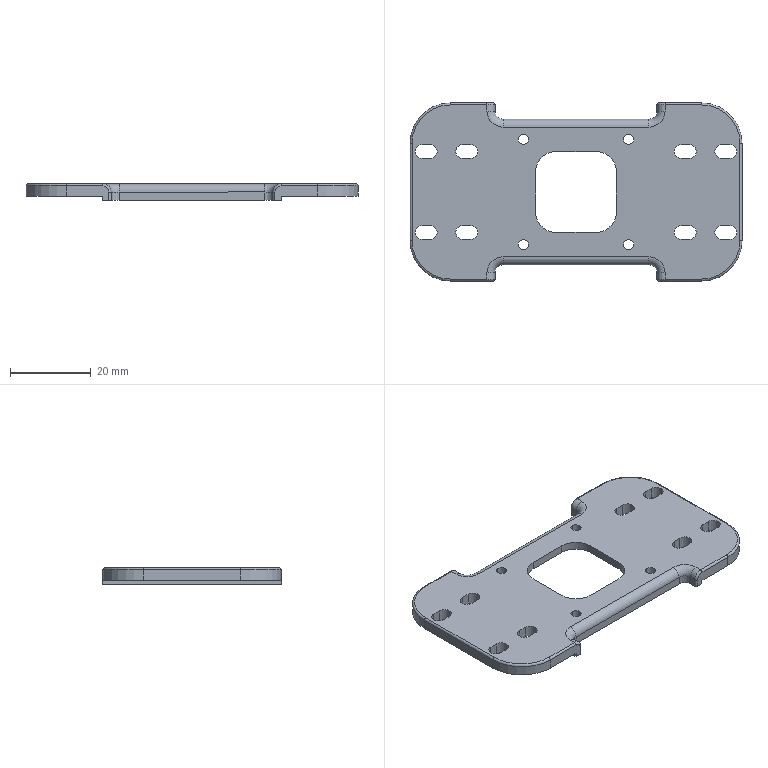NC program | NX | posted with a generic post | part box 82 x 44 x 4 mm
Lines 4216 to 5497 of 6362:
(ZLEVEL_PROFILE_1_COPY_COPY_COPY , TOOL : D3R0.5)
N8388 T18 M6
N8390 G54
N8392 G17 G0 G90 X19.987 Y23.676 S9500 M3
N8394 G43 Z30. H18
N8396 Z2.984
N8398 G94 G1 Z-0.016 F1000.
N8400 G3 X21.508 Y22.645 R1.5
N8402 G1 X22. Y22.677 F2500.
N8404 X31.
N8406 G2 X41.677 Y12. R10.677
N8408 G1 Y-12.
N8410 G2 X31. Y-22.677 R10.677
N8412 G1 X22.
N8414 X21.509 Y-22.646
N8416 X21.503 Y-22.724 Z-0.028
N8418 X21.5 Y-22.767 Z-0.04
N8420 X21.538 Y-22.762
N8422 X22. Y-22.78
N8424 X31.
N8426 G3 X41.78 Y-12. R10.78
N8428 G1 Y12.
N8430 G3 X31. Y22.78 R10.78
N8432 G1 X22.
N8434 X21.519 Y22.762
N8436 X21.509 Y22.764
N8438 X21.504 Y22.822 Z-0.057
N8440 X21.5 Y22.862 Z-0.074
N8442 X22. Y22.876
N8444 X31.
N8446 G2 X41.876 Y12. R10.876
N8448 G1 Y-12.
N8450 G2 X31. Y-22.876 R10.876
N8452 G1 X22.
N8454 X21.538 Y-22.863
N8456 X21.5 Y-22.862
N8458 Y-22.92 Z-0.095
N8460 Y-22.959 Z-0.116
N8462 X22. Y-22.968
N8464 X31.
N8466 G3 X41.968 Y-12. R10.968
N8468 G1 Y12.
N8470 G3 X31. Y22.968 R10.968
N8472 G1 X22.
N8474 X21.5 Y22.959
N8476 Y23.004 Z-0.142
N8478 Y23.049 Z-0.168
N8480 X22. Y23.055
N8482 X31.
N8484 G2 X42.055 Y12. R11.055
N8486 G1 Y-12.
N8488 G2 X31. Y-23.055 R11.055
N8490 G1 X22.
N8492 X21.5 Y-23.049
N8494 Y-23.093 Z-0.198
N8496 Y-23.127 Z-0.228
N8498 X22. Y-23.136
N8500 X31.
N8502 G3 X42.136 Y-12. R11.136
N8504 G1 Y12.
N8506 G3 X31. Y23.136 R11.136
N8508 G1 X22.
N8510 X21.5 Y23.127
N8512 Y23.168 Z-0.262
N8514 Y23.2 Z-0.296
N8516 X22. Y23.21
N8518 X31.
N8520 G2 X42.21 Y12. R11.21
N8522 G1 Y-12.
N8524 G2 X31. Y-23.21 R11.21
N8526 G1 X22.
N8528 X21.5 Y-23.2
N8530 Y-23.237 Z-0.333
N8532 Y-23.269 Z-0.37
N8534 X22. Y-23.277
N8536 X31.
N8538 G3 X42.277 Y-12. R11.277
N8540 G1 Y12.
N8542 G3 X31. Y23.277 R11.277
N8544 G1 X22.
N8546 X21.5 Y23.269
N8548 X21.416 Y23.323 Z-0.451
N8550 G2 X22. Y23.336 R15.223
N8552 G1 X31.
N8554 G2 X42.336 Y12. R11.336
N8556 G1 Y-12.
N8558 G2 X31. Y-23.336 R11.336
N8560 G1 X22.
N8562 X21.416 Y-23.325
N8564 Y-23.354 Z-0.495
N8566 Y-23.375 Z-0.538
N8568 X22. Y-23.387
N8570 X31.
N8572 G3 X42.387 Y-12. R11.387
N8574 G1 Y12.
N8576 G3 X31. Y23.387 R11.387
N8578 G1 X22.
N8580 G3 X21.416 Y23.373 R27.173
N8582 G1 Y23.4 Z-0.583
N8584 Y23.415 Z-0.629
N8586 X22. Y23.429
N8588 X31.
N8590 G2 X42.429 Y12. R11.429
N8592 G1 Y-12.
N8594 G2 X31. Y-23.429 R11.429
N8596 G1 X22.
N8598 X21.416 Y-23.417
N8600 Y-23.436 Z-0.675
N8602 Y-23.449 Z-0.722
N8604 X22. Y-23.46
N8606 X31.
N8608 G3 X42.46 Y-12. R11.46
N8610 G1 Y12.
N8612 G3 X31. Y23.46 R11.46
N8614 G1 X22.
N8616 X21.416 Y23.449
N8618 Y23.465 Z-0.768
N8620 Y23.471 Z-0.814
N8622 X22. Y23.483
N8624 X31.
N8626 G2 X42.483 Y12. R11.483
N8628 G1 Y-12.
N8630 G2 X31. Y-23.483 R11.483
N8632 G1 X22.
N8634 X21.416 Y-23.471
N8636 Y-23.481 Z-0.861
N8638 Y-23.485 Z-0.907
N8640 X22. Y-23.496
N8642 X31.
N8644 G3 X42.496 Y-12. R11.496
N8646 G1 Y12.
N8648 G3 X31. Y23.496 R11.496
N8650 G1 X22.
N8652 X21.416 Y23.485
N8654 Y23.492 Z-1.
N8656 X21.538 Y23.497
N8658 X31.055 Y23.498
N8660 G2 X42.5 Y12. R11.499
N8662 G1 Y-11.824
N8664 X42.499 Y-12.068
N8666 G2 X31.055 Y-23.498 R11.498
N8668 G1 X21.538 Y-23.497
N8670 X21.416 Y-23.492
N8672 G3 X19.883 Y-24.73 R1.5
N8674 G1 Z2.
N8676 G0 Z30.
N8678 X-20.168 Y-23.794
N8680 Z2.984
N8682 G1 Z-0.016 F1000.
N8684 X-20.991 Y-22.892
N8686 G3 X-21.51 Y-22.649 R0.75
N8688 G1 X-21.537 Y-22.663 F2500.
N8690 X-22. Y-22.677
N8692 X-31.
N8694 G2 X-41.677 Y-12. R10.677
N8696 G1 Y12.
N8698 G2 X-31. Y22.677 R10.677
N8700 G1 X-22.
N8702 X-21.508 Y22.643
N8704 Y22.705 Z-0.028
N8706 Y22.764 Z-0.04
N8708 X-21.518 Y22.761
N8710 X-22. Y22.78
N8712 X-31.
N8714 G3 X-41.78 Y12. R10.78
N8716 G1 Y-12.
N8718 G3 X-31. Y-22.78 R10.78
N8720 G1 X-22.
N8722 X-21.518 Y-22.761
N8724 X-21.508 Y-22.764
N8726 X-21.503 Y-22.822 Z-0.057
N8728 X-21.5 Y-22.862 Z-0.074
N8730 X-22. Y-22.876
N8732 X-31.
N8734 G2 X-41.876 Y-12. R10.876
N8736 G1 Y12.
N8738 G2 X-31. Y22.876 R10.876
N8740 G1 X-22.
N8742 X-21.538 Y22.863
N8744 X-21.5 Y22.862
N8746 Y22.919 Z-0.095
N8748 Y22.959 Z-0.116
N8750 X-22. Y22.968
N8752 X-31.
N8754 G3 X-41.968 Y12. R10.968
N8756 G1 Y-12.
N8758 G3 X-31. Y-22.968 R10.968
N8760 G1 X-22.
N8762 X-21.5 Y-22.959
N8764 Y-23.008 Z-0.142
N8766 Y-23.049 Z-0.168
N8768 X-22. Y-23.055
N8770 X-31.
N8772 G2 X-42.055 Y-12. R11.055
N8774 G1 Y12.
N8776 G2 X-31. Y23.055 R11.055
N8778 G1 X-22.
N8780 X-21.5 Y23.049
N8782 Y23.093 Z-0.198
N8784 Y23.127 Z-0.228
N8786 X-22. Y23.136
N8788 X-31.
N8790 G3 X-42.136 Y12. R11.136
N8792 G1 Y-12.
N8794 G3 X-31. Y-23.136 R11.136
N8796 G1 X-22.
N8798 X-21.5 Y-23.127
N8800 Y-23.168 Z-0.262
N8802 Y-23.2 Z-0.296
N8804 X-22. Y-23.21
N8806 X-31.
N8808 G2 X-42.21 Y-12. R11.21
N8810 G1 Y12.
N8812 G2 X-31. Y23.21 R11.21
N8814 G1 X-22.
N8816 X-21.5 Y23.2
N8818 Y23.237 Z-0.333
N8820 Y23.269 Z-0.37
N8822 X-22. Y23.277
N8824 X-31.
N8826 G3 X-42.277 Y12. R11.277
N8828 G1 Y-12.
N8830 G3 X-31. Y-23.277 R11.277
N8832 G1 X-22.
N8834 X-21.5 Y-23.269
N8836 Y-23.305 Z-0.411
N8838 Y-23.333 Z-0.451
N8840 X-22. Y-23.336
N8842 X-31.
N8844 G2 X-42.336 Y-12. R11.336
N8846 G1 Y12.
N8848 G2 X-31. Y23.336 R11.336
N8850 G1 X-22.
N8852 X-21.5 Y23.333
N8854 Y23.359 Z-0.495
N8856 Y23.381 Z-0.538
N8858 X-22. Y23.387
N8860 X-31.
N8862 G3 X-42.387 Y12. R11.387
N8864 G1 Y-12.
N8866 G3 X-31. Y-23.387 R11.387
N8868 G1 X-22.
N8870 X-21.5 Y-23.381
N8872 Y-23.406 Z-0.583
N8874 Y-23.424 Z-0.629
N8876 X-22. Y-23.429
N8878 X-31.
N8880 G2 X-42.429 Y-12. R11.429
N8882 G1 Y12.
N8884 G2 X-31. Y23.429 R11.429
N8886 G1 X-22.
N8888 X-21.5 Y23.424
N8890 Y23.439 Z-0.675
N8892 Y23.453 Z-0.722
N8894 X-21.538 Y23.455
N8896 X-22. Y23.46
N8898 X-31.
N8900 G3 X-42.46 Y12. R11.46
N8902 G1 Y-12.
N8904 G3 X-31. Y-23.46 R11.46
N8906 G1 X-22.
N8908 X-21.538 Y-23.455
N8910 X-21.5 Y-23.453
N8912 Y-23.47 Z-0.768
N8914 Y-23.48 Z-0.814
N8916 X-22. Y-23.483
N8918 X-31.
N8920 G2 X-42.483 Y-12. R11.483
N8922 G1 Y12.
N8924 G2 X-31. Y23.483 R11.483
N8926 G1 X-22.
N8928 X-21.474 Y23.479
N8930 X-21.416 Y23.485 Z-0.907
N8932 X-22. Y23.496
N8934 X-31.
N8936 G3 X-42.496 Y12. R11.496
N8938 G1 Y-12.
N8940 G3 X-31. Y-23.496 R11.496
N8942 G1 X-22.
N8944 X-21.416 Y-23.485
N8946 Y-23.492 Z-1.
N8948 X-21.538 Y-23.497
N8950 X-31.055 Y-23.498
N8952 G2 X-42.498 Y-12.068 R11.498
N8954 G1 Y11.998
N8956 G2 X-30.996 Y23.498 R11.501
N8958 G1 X-21.538 Y23.497
N8960 X-21.416 Y23.492
N8962 G3 X-19.876 Y24.727 R1.5
N8964 G1 Z2.
N8966 G0 Z30.
(ZLEVEL_PROFILE_1_COPY_COPY_COPY_COPY , TOOL : D3R0.5)
N8968 X-23.155 Y24.133
N8970 Z2.991
N8972 G1 Z-0.009 F1000.
N8974 G3 X-21.996 Y22.622 R1.5
N8976 G2 X-20.789 Y21.5 R1.325 F2500.
N8978 G1 Y20.
N8980 G3 X-18. Y17.211 R2.789
N8982 G1 X18.
N8984 G3 X20.789 Y20. R2.789
N8986 G1 Y21.5
N8988 G2 X22. Y22.633 R1.251
N8990 G1 Y22.665 Z-0.015
N8992 Y22.705 Z-0.021
N8994 G3 X20.674 Y21.5 R1.339
N8996 G1 Y20.
N8998 G2 X18. Y17.326 R2.674
N9000 G1 X-18.
N9002 G2 X-20.674 Y20. R2.674
N9004 G1 Y21.5
N9006 G3 X-21.998 Y22.695 R1.318
N9008 G1 X-21.975 Y22.771 Z-0.038
N9010 G2 X-20.567 Y21.5 R1.409
N9012 G1 Y20.
N9014 G3 X-18. Y17.433 R2.567
N9016 G1 X18.
N9018 G3 X20.567 Y20. R2.567
N9020 G1 Y21.5
N9022 G2 X21.968 Y22.771 R1.406
N9024 G1 X21.912 Y22.826 Z-0.058
N9026 G3 X20.464 Y21.5 R1.458
N9028 G1 Y20.
N9030 G2 X18. Y17.536 R2.464
N9032 G1 X-18.
N9034 G2 X-20.464 Y20. R2.464
N9036 G1 Y21.5
N9038 G3 X-21.92 Y22.826 R1.455
N9040 G1 X-21.921 Y22.862 Z-0.07
N9042 Y22.89 Z-0.082
N9044 G2 X-20.363 Y21.5 R1.525
N9046 G1 Y20.
N9048 G3 X-18. Y17.637 R2.363
N9050 G1 X18.
N9052 G3 X20.363 Y20. R2.363
N9054 G1 Y21.5
N9056 G2 X22. Y22.898 R1.558
N9058 G1 X22.002 Y22.928 Z-0.096
N9060 X22.003 Y22.952 Z-0.111
N9062 G3 X21.477 Y22.876 R1.681
N9064 G1 X21.136 Y22.77
N9066 G3 X20.265 Y21.5 R1.494
N9068 G1 Y20.
N9070 G2 X18. Y17.735 R2.265
N9072 G1 X-18.
N9074 G2 X-20.265 Y20. R2.265
N9076 G1 Y21.5
N9078 G3 X-21.922 Y22.946 R1.625
N9080 G1 X-22. Y23.014 Z-0.142
N9082 G2 X-20.624 Y22.501 R2.093
N9084 X-20.168 Y21.501 R1.325
N9086 G1 Y20.
N9088 G3 X-18. Y17.832 R2.168
N9090 G1 X18.
N9092 G3 X20.168 Y20. R2.168
N9094 G1 Y21.5
N9096 G2 X21.091 Y22.814 R1.513
N9098 G1 X21.335 Y22.897
N9100 G2 X22. Y23.014 R1.94
N9102 G1 Y23.041 Z-0.16
N9104 Y23.07 Z-0.178
N9106 G3 X20.629 Y22.61 R2.309
N9108 X20.073 Y21.5 R1.386
N9110 G1 Y20.
N9112 G2 X18. Y17.927 R2.073
N9114 G1 X-18.
N9116 G2 X-20.073 Y20. R2.073
N9118 G1 Y21.502
N9120 G3 X-20.628 Y22.614 R1.391
N9122 X-22. Y23.069 R2.271
N9124 G1 Y23.097 Z-0.198
N9126 Y23.123 Z-0.218
N9128 G2 X-20.723 Y22.77 R2.491
N9130 X-19.98 Y21.5 R1.565
N9132 G1 Y20.
N9134 G3 X-18. Y18.02 R1.98
N9136 G1 X18.
N9138 G3 X19.98 Y20. R1.98
N9140 G1 Y21.5
N9142 G2 X20.847 Y22.846 R1.597
N9144 X22. Y23.123 R2.641
N9146 G1 Y23.147 Z-0.239
N9148 Y23.173 Z-0.261
N9150 G3 X20.847 Y22.918 R2.781
N9152 X19.889 Y21.5 R1.637
N9154 G1 Y20.
N9156 G2 X18. Y18.111 R1.889
N9158 G1 X-18.
N9160 G2 X-19.889 Y20. R1.889
N9162 G1 Y21.5
N9164 G3 X-20.847 Y22.918 R1.637
N9166 X-22. Y23.173 R2.78
N9168 G1 Y23.198 Z-0.284
N9170 Y23.218 Z-0.307
N9172 G2 X-20.847 Y22.984 R2.953
N9174 X-19.799 Y21.5 R1.688
N9176 G1 Y20.
N9178 G3 X-18. Y18.201 R1.799
N9180 G1 X18.
N9182 G3 X19.799 Y20. R1.799
N9184 G1 Y21.5
N9186 G2 X20.847 Y22.984 R1.688
N9188 X22. Y23.221 R3.054
N9190 G1 X22.001 Y23.244 Z-0.332
N9192 Y23.266 Z-0.357
N9194 G3 X20.775 Y23.014 R3.086
N9196 X19.712 Y21.5 R1.719
N9198 G1 Y20.
N9200 G2 X18. Y18.288 R1.712
N9202 G1 X-18.
N9204 G2 X-19.712 Y20. R1.712
N9206 G1 Y21.5
N9208 G3 X-20.775 Y23.014 R1.719
N9210 X-22.001 Y23.266 R3.086
N9212 G1 Y23.286 Z-0.384
N9214 Y23.307 Z-0.411
N9216 G2 X-20.643 Y23.014 R3.157
N9218 X-19.627 Y21.5 R1.753
N9220 G1 Y20.
N9222 G3 X-18. Y18.373 R1.627
N9224 G1 X18.
N9226 G3 X19.627 Y20. R1.627
N9228 G1 Y21.5
N9230 G2 X20.643 Y23.014 R1.753
N9232 X22.001 Y23.307 R3.157
N9234 G1 X22. Y23.328 Z-0.439
N9236 Y23.345 Z-0.468
N9238 G3 X20.523 Y23.014 R3.134
N9240 X19.544 Y21.5 R1.763
N9242 G1 Y20.
N9244 G2 X18. Y18.456 R1.544
N9246 G1 X-18.
N9248 G2 X-19.544 Y20. R1.544
N9250 G1 Y21.5
N9252 G3 X-20.523 Y23.014 R1.763
N9254 X-22. Y23.345 R3.134
N9256 G1 Y23.365 Z-0.498
N9258 Y23.381 Z-0.528
N9260 G2 X-20.603 Y23.117 R3.547
N9262 X-19.463 Y21.5 R1.844
N9264 G1 Y20.
N9266 G3 X-18. Y18.537 R1.463
N9268 G1 X18.
N9270 G3 X19.463 Y20. R1.463
N9272 G1 Y21.5
N9274 G2 X20.603 Y23.117 R1.844
N9276 X22. Y23.381 R3.547
N9278 G1 X21.999 Y23.395 Z-0.56
N9280 Y23.41 Z-0.591
N9282 G3 X20.603 Y23.168 R3.688
N9284 X19.385 Y21.5 R1.872
N9286 G1 Y20.
N9288 G2 X18. Y18.615 R1.385
N9290 G1 X-18.
N9292 G2 X-19.385 Y20. R1.385
N9294 G1 Y21.5
N9296 G3 X-20.603 Y23.168 R1.872
N9298 X-21.999 Y23.41 R3.688
N9300 G1 Y23.423 Z-0.624
N9302 Y23.439 Z-0.658
N9304 G2 X-20.716 Y23.258 R4.282
N9306 X-19.628 Y22.482 R2.119
N9308 X-19.31 Y21.5 R1.862
N9310 G1 Y20.
N9312 G3 X-18. Y18.69 R1.31
N9314 G1 X18.
N9316 G3 X19.31 Y20. R1.31
N9318 G1 Y21.5
N9320 G2 X20.198 Y23.014 R1.821
N9322 X21.091 Y23.356 R2.685
N9324 X21.999 Y23.439 R5.278
N9326 G1 X21.998 Y23.446 Z-0.692
N9328 Y23.461 Z-0.727
N9330 G3 X21.091 Y23.388 R5.523
N9332 X20.116 Y23.025 R2.68
N9334 X19.238 Y21.5 R1.859
N9336 G1 Y20.
N9338 G2 X18. Y18.762 R1.238
N9340 G1 X-18.
N9342 G2 X-19.238 Y20. R1.238
N9344 G1 Y21.5
N9346 G3 X-19.581 Y22.526 R1.843
N9348 X-20.663 Y23.281 R2.102
N9350 X-21.998 Y23.461 R4.326
N9352 G1 Y23.47 Z-0.763
N9354 Y23.476 Z-0.799
N9356 G2 X-20.919 Y23.385 R5.203
N9358 X-20.012 Y23.014 R2.608
N9360 X-19.168 Y21.5 R1.862
N9362 G1 Y20.
N9364 G3 X-18. Y18.832 R1.168
N9366 G1 X18.
N9368 G3 X19.168 Y20. R1.168
N9370 G1 Y21.5
N9372 G2 X20.012 Y23.014 R1.862
N9374 X21.011 Y23.402 R2.592
N9376 X21.998 Y23.476 R5.171
N9378 G1 Y23.483 Z-0.836
N9380 Y23.488 Z-0.874
N9382 G3 X21.011 Y23.429 R6.639
N9384 X19.923 Y23.014 R2.496
N9386 X19.101 Y21.5 R1.888
N9388 G1 Y20.
N9390 G2 X18. Y18.899 R1.101
N9392 G1 X-18.
N9394 G2 X-19.101 Y20. R1.101
N9396 G1 Y21.5
N9398 G3 X-19.63 Y22.77 R1.918
N9400 X-21.011 Y23.429 R2.413
N9402 X-21.998 Y23.488 R6.645
N9404 G1 X-22.005 Y23.5 Z-0.951
N9406 X-21.26 Y23.475
N9408 G2 X-20.116 Y23.176 R2.803
N9410 X-19.038 Y21.5 R1.913
N9412 G1 Y20.
N9414 G3 X-18. Y18.962 R1.038
N9416 G1 X18.
N9418 G3 X19.038 Y20. R1.038
N9420 G1 Y21.5
N9422 G2 X19.872 Y23.034 R1.911
N9424 G1 X20.012 Y23.116
N9426 G2 X21.141 Y23.466 R2.637
N9428 G1 X21.261 Y23.475
N9430 X22.005 Y23.5
N9432 X21.898 Y23.499 Z-0.978
N9434 X21.792 Y23.5 Z-1.004
N9436 X21.685 Z-1.031
N9438 X21.091 Y23.475
N9440 G3 X19.765 Y23.014 R2.643
N9442 X18.977 Y21.5 R1.921
N9444 G1 Y20.
N9446 G2 X18. Y19.023 R0.977
N9448 G1 X-18.
N9450 G2 X-18.977 Y20. R0.977
N9452 G1 Y21.5
N9454 G3 X-19.765 Y23.014 R1.921
N9456 X-20.926 Y23.456 R2.562
N9458 X-21.685 Y23.5 R6.251
N9460 G1 X-21.417 Z-1.113
N9462 G2 X-20.442 Y23.38 R3.773
N9464 X-19.14 Y22.367 R2.115
N9466 X-18.92 Y21.5 R2.
N9468 G1 Y20.
N9470 G3 X-18. Y19.08 R0.92
N9472 G1 X18.
N9474 G3 X18.92 Y20. R0.92
N9476 G1 Y21.5
N9478 G2 X19.697 Y23.014 R1.932
N9480 X20.721 Y23.443 R2.38
N9482 G1 X20.847 Y23.465
N9484 X21.417 Y23.5
N9486 X21.261 Z-1.198
N9488 G3 X20.033 Y23.258 R2.93
N9490 X18.866 Y21.5 R1.972
N9492 G1 Y20.
N9494 G2 X18. Y19.134 R0.866
N9496 G1 X-18.
N9498 G2 X-18.866 Y20. R0.866
N9500 G1 Y21.5
N9502 G3 X-20.033 Y23.258 R1.972
N9504 X-21.259 Y23.5 R2.929
N9506 G1 X-21.12 Z-1.284
N9508 G2 X-19.872 Y23.211 R2.671
N9510 X-18.816 Y21.5 R1.977
N9512 G1 Y20.
N9514 G3 X-18. Y19.184 R0.816
N9516 G1 X18.
N9518 G3 X18.816 Y20. R0.816
N9520 G1 Y21.5
N9522 G2 X19.964 Y23.258 R1.987
N9524 G1 X20.116 Y23.319
N9526 G2 X21.12 Y23.5 R2.649
N9528 G1 X21.01 Z-1.373
N9530 G3 X19.872 Y23.243 R2.6
N9532 X18.769 Y21.5 R1.984
N9534 G1 Y20.
N9536 G2 X18. Y19.231 R0.769
N9538 G1 X-18.
N9540 G2 X-18.769 Y20. R0.769
N9542 G1 Y21.5
N9544 G3 X-19.872 Y23.243 R1.984
N9546 X-21.01 Y23.5 R2.6
N9548 G1 X-20.917 Z-1.463
N9550 G2 X-19.845 Y23.258 R2.479
N9552 X-18.725 Y21.5 R1.984
N9554 G1 Y20.
N9556 G3 X-18. Y19.275 R0.725
N9558 G1 X18.
N9560 G3 X18.725 Y20. R0.725
N9562 G1 Y21.5
N9564 G2 X19.845 Y23.258 R1.984
N9566 X20.917 Y23.5 R2.479
N9568 G1 X20.835 Z-1.555
N9570 G3 X19.872 Y23.294 R2.417
N9572 X18.686 Y21.5 R1.987
N9574 G1 Y20.
N9576 G2 X18. Y19.314 R0.686
N9578 G1 X-18.
N9580 G2 X-18.686 Y20. R0.686
N9582 G1 Y21.5
N9584 G3 X-19.872 Y23.294 R1.987
N9586 X-20.835 Y23.5 R2.417
N9588 G1 X-20.763 Z-1.648
N9590 G2 X-20.116 Y23.405 R2.44
N9592 X-18.65 Y21.5 R2.011
N9594 G1 Y20.
N9596 G3 X-18. Y19.35 R0.65
N9598 G1 X18.
N9600 G3 X18.65 Y20. R0.65
N9602 G1 Y21.5
N9604 G2 X19.872 Y23.317 R2.003
N9606 X20.763 Y23.5 R2.301
N9608 G1 X20.72 Z-1.736
N9610 G3 X19.872 Y23.335 R2.288
N9612 X18.62 Y21.5 R2.016
N9614 G1 Y20.
N9616 G2 X18. Y19.38 R0.62
N9618 G1 X-18.
N9620 G2 X-18.62 Y20. R0.62
N9622 G1 Y21.5
N9624 G3 X-18.914 Y22.526 R2.096
N9626 X-20.72 Y23.5 R2.104
N9628 G1 X-20.657 Z-1.824
N9630 G2 X-18.896 Y22.543 R2.077
N9632 X-18.593 Y21.5 R2.044
N9634 G1 Y20.
N9636 G3 X-18. Y19.407 R0.593
N9638 G1 X18.
N9640 G3 X18.593 Y20. R0.593
N9642 G1 Y21.5
N9644 G2 X19.872 Y23.35 R2.016
N9646 G1 X20.037 Y23.403
N9648 G2 X20.657 Y23.5 R2.015
N9650 G1 X20.615 Z-1.912
N9652 G3 X18.57 Y21.5 R2.029
N9654 G1 Y20.
N9656 G2 X18. Y19.43 R0.57
N9658 G1 X-18.
N9660 G2 X-18.57 Y20. R0.57
N9662 G1 Y21.5
N9664 G3 X-20.615 Y23.5 R2.029
N9666 G1 X-20.582 Z-2.
N9668 G2 X-18.84 Y22.526 R2.053
N9670 X-18.551 Y21.5 R2.077
N9672 G1 Y20.
N9674 G3 X-18. Y19.449 R0.551
N9676 G1 X18.
N9678 G3 X18.551 Y20. R0.551
N9680 G1 Y21.5
N9682 G2 X20.582 Y23.5 R2.026
N9684 G3 X22.086 Y25. R1.5
N9686 G1 Z1.
N9688 G0 Z30.
N9690 X23.142 Y-24.133
N9692 Z2.991
N9694 G1 Z-0.009 F1000.
N9696 G3 X21.999 Y-22.624 R1.5
N9698 G2 X20.789 Y-21.5 R1.337 F2500.
N9700 G1 Y-20.
N9702 G3 X18. Y-17.211 R2.789
N9704 G1 X-18.
N9706 G3 X-20.789 Y-20. R2.789
N9708 G1 Y-21.5
N9710 G2 X-21.92 Y-22.614 R1.182
N9712 G1 X-21.918 Y-22.662 Z-0.015
N9714 Y-22.69 Z-0.021
N9716 G3 X-20.674 Y-21.5 R1.307
N9718 G1 Y-20.
N9720 G2 X-18. Y-17.326 R2.674
N9722 G1 X18.
N9724 G2 X20.674 Y-20. R2.674
N9726 G1 Y-21.5
N9728 G3 X22.003 Y-22.698 R1.324
N9730 G1 X22.001 Y-22.741 Z-0.03
N9732 X22. Y-22.772 Z-0.038
N9734 G2 X20.567 Y-21.5 R1.41
N9736 G1 Y-20.
N9738 G3 X18. Y-17.433 R2.567
N9740 G1 X-18.
N9742 G3 X-20.567 Y-20. R2.567
N9744 G1 Y-21.5
N9746 G2 X-22. Y-22.772 R1.413
N9748 G1 X-21.999 Y-22.806 Z-0.048
N9750 Y-22.833 Z-0.058
N9752 G3 X-20.464 Y-21.5 R1.525
N9754 G1 Y-20.
N9756 G2 X-18. Y-17.536 R2.464
N9758 G1 X18.
N9760 G2 X20.464 Y-20. R2.464
N9762 G1 Y-21.5
N9764 G3 X21.999 Y-22.836 R1.453
N9766 G1 X22. Y-22.868 Z-0.07
N9768 Y-22.898 Z-0.082
N9770 G2 X20.363 Y-21.5 R1.558
N9772 G1 Y-20.
N9774 G3 X18. Y-17.637 R2.363
N9776 G1 X-18.
N9778 G3 X-20.363 Y-20. R2.363
N9780 G1 Y-21.5
N9782 G2 X-21.999 Y-22.895 R1.606
N9784 G1 Y-22.928 Z-0.096
N9786 X-22. Y-22.957 Z-0.111
N9788 G3 X-21.461 Y-22.871 R1.901
N9790 G1 X-21.136 Y-22.77
N9792 G3 X-20.265 Y-21.5 R1.494
N9794 G1 Y-20.
N9796 G2 X-18. Y-17.735 R2.265
N9798 G1 X18.
N9800 G2 X20.265 Y-20. R2.265
N9802 G1 Y-21.501
N9804 G3 X20.549 Y-22.291 R1.243
N9806 X22. Y-22.952 R1.818
N9808 G1 Y-22.987 Z-0.127
N9810 Y-23.014 Z-0.142
N9812 G2 X20.624 Y-22.501 R2.095
N9814 X20.168 Y-21.501 R1.324
N9816 G1 Y-20.
N9818 G3 X18. Y-17.832 R2.168
N9820 G1 X-18.
N9822 G3 X-20.168 Y-20. R2.168
N9824 G1 Y-21.5
N9826 G2 X-21.091 Y-22.814 R1.513
N9828 G1 X-21.335 Y-22.897
N9830 G2 X-21.997 Y-23.014 R1.932
N9832 G1 X-22.001 Y-23.043 Z-0.16
N9834 X-22.005 Y-23.069 Z-0.178
N9836 G3 X-20.617 Y-22.6 R2.292
N9838 X-20.073 Y-21.5 R1.382
N9840 G1 Y-20.
N9842 G2 X-18. Y-17.927 R2.073
N9844 G1 X18.
N9846 G2 X20.073 Y-20. R2.073
N9848 G1 Y-21.5
N9850 G3 X20.633 Y-22.617 R1.394
N9852 X22. Y-23.07 R2.277
N9854 G1 Y-23.095 Z-0.198
N9856 Y-23.123 Z-0.218
N9858 G2 X20.723 Y-22.77 R2.473
N9860 X19.98 Y-21.5 R1.565
N9862 G1 Y-20.
N9864 G3 X18. Y-18.02 R1.98
N9866 G1 X-18.
N9868 G3 X-19.98 Y-20. R1.98
N9870 G1 Y-21.5
N9872 G2 X-20.847 Y-22.846 R1.596
N9874 X-22. Y-23.123 R2.673
N9876 G1 Y-23.147 Z-0.239
N9878 Y-23.173 Z-0.261
N9880 G3 X-20.847 Y-22.918 R2.78
N9882 X-19.889 Y-21.5 R1.636
N9884 G1 Y-20.
N9886 G2 X-18. Y-18.111 R1.889
N9888 G1 X18.
N9890 G2 X19.889 Y-20. R1.889
N9892 G1 Y-21.5
N9894 G3 X20.847 Y-22.918 R1.636
N9896 X22. Y-23.173 R2.781
N9898 G1 Y-23.196 Z-0.284
N9900 Y-23.221 Z-0.307
N9902 G2 X20.847 Y-22.984 R3.054
N9904 X19.799 Y-21.5 R1.688
N9906 G1 Y-20.
N9908 G3 X18. Y-18.201 R1.799
N9910 G1 X-18.
N9912 G3 X-19.799 Y-20. R1.799
N9914 G1 Y-21.5
N9916 G2 X-20.847 Y-22.984 R1.688
N9918 X-22.024 Y-23.219 R2.995
N9920 G1 X-22.001 Y-23.266 Z-0.357
N9922 G3 X-20.775 Y-23.014 R3.087
N9924 X-19.712 Y-21.5 R1.718
N9926 G1 Y-20.
N9928 G2 X-18. Y-18.288 R1.712
N9930 G1 X18.
N9932 G2 X19.712 Y-20. R1.712
N9934 G1 Y-21.5
N9936 G3 X20.775 Y-23.014 R1.718
N9938 X22. Y-23.266 R3.085
N9940 G1 Y-23.288 Z-0.384
N9942 Y-23.307 Z-0.411
N9944 G2 X20.643 Y-23.014 R3.156
N9946 X19.627 Y-21.5 R1.753
N9948 G1 Y-20.
N9950 G3 X18. Y-18.373 R1.627
N9952 G1 X-18.
N9954 G3 X-19.627 Y-20. R1.627
N9956 G1 Y-21.5
N9958 G2 X-20.643 Y-23.014 R1.753
N9960 X-22. Y-23.307 R3.157
N9962 G1 X-21.999 Y-23.328 Z-0.439
N9964 Y-23.345 Z-0.468
N9966 G3 X-20.523 Y-23.014 R3.133
N9968 X-19.544 Y-21.5 R1.763
N9970 G1 Y-20.
N9972 G2 X-18. Y-18.456 R1.544
N9974 G1 X18.
N9976 G2 X19.544 Y-20. R1.544
N9978 G1 Y-21.5
N9980 G3 X20.523 Y-23.014 R1.763
N9982 X21.999 Y-23.345 R3.133
N9984 G1 Y-23.362 Z-0.498
N9986 Y-23.381 Z-0.528
N9988 G2 X20.603 Y-23.117 R3.546
N9990 X19.463 Y-21.5 R1.844
N9992 G1 Y-20.
N9994 G3 X18. Y-18.537 R1.463
N9996 G1 X-18.
N9998 G3 X-19.463 Y-20. R1.463
N10000 G1 Y-21.5
N10002 G2 X-20.603 Y-23.117 R1.844
N10004 X-21.998 Y-23.381 R3.546
N10006 G1 Y-23.395 Z-0.56
N10008 X-21.997 Y-23.41 Z-0.591
N10010 G3 X-20.603 Y-23.168 R3.684
N10012 X-19.385 Y-21.5 R1.872
N10014 G1 Y-20.
N10016 G2 X-18. Y-18.615 R1.385
N10018 G1 X18.
N10020 G2 X19.385 Y-20. R1.385
N10022 G1 Y-21.5
N10024 G3 X20.603 Y-23.168 R1.872
N10026 X21.998 Y-23.41 R3.686
N10028 G1 Y-23.423 Z-0.624
N10030 Y-23.439 Z-0.658
N10032 G2 X20.752 Y-23.267 R4.168
N10034 X19.628 Y-22.482 R2.171
N10036 X19.31 Y-21.5 R1.862
N10038 G1 Y-20.
N10040 G3 X18. Y-18.69 R1.31
N10042 G1 X-18.
N10044 G3 X-19.31 Y-20. R1.31
N10046 G1 Y-21.5
N10048 G2 X-20.198 Y-23.014 R1.821
N10050 X-21.091 Y-23.356 R2.684
N10052 X-21.997 Y-23.439 R5.279
N10054 G1 Y-23.446 Z-0.692
N10056 X-21.996 Y-23.461 Z-0.727
N10058 G3 X-21.091 Y-23.388 R5.521
N10060 X-20.116 Y-23.025 R2.682
N10062 X-19.238 Y-21.5 R1.859
N10064 G1 Y-20.
N10066 G2 X-18. Y-18.762 R1.238
N10068 G1 X18.
N10070 G2 X19.238 Y-20. R1.238
N10072 G1 Y-21.503
N10074 G3 X19.44 Y-22.295 R1.648
N10076 X20.585 Y-23.258 R2.066
N10078 X21.998 Y-23.461 R4.353
N10080 G1 Y-23.47 Z-0.763
N10082 Y-23.476 Z-0.799
N10084 G2 X20.919 Y-23.385 R5.203
N10086 X19.872 Y-22.911 R2.506
N10088 X19.168 Y-21.5 R1.854
N10090 G1 Y-20.
N10092 G3 X18. Y-18.832 R1.168
N10094 G1 X-18.
N10096 G3 X-19.168 Y-20. R1.168
N10098 G1 Y-21.5
N10100 G2 X-20.012 Y-23.014 R1.862
N10102 X-21.011 Y-23.402 R2.571
N10104 X-21.996 Y-23.476 R5.163
N10106 G1 Y-23.483 Z-0.836
N10108 Y-23.488 Z-0.874
N10110 G3 X-21.091 Y-23.441 R7.578
N10112 X-20.116 Y-23.134 R2.821
N10114 X-19.101 Y-21.5 R1.905
N10116 G1 Y-20.
N10118 G2 X-18. Y-18.899 R1.101
N10120 G1 X18.
N10122 G2 X19.101 Y-20. R1.101
N10124 G1 Y-21.5
N10126 G3 X20.116 Y-23.134 R1.905
N10128 X21.011 Y-23.429 R2.733
N10130 X21.998 Y-23.488 R6.644
N10132 G1 X22.005 Y-23.5 Z-0.951
N10134 X21.26 Y-23.475
N10136 G2 X20.116 Y-23.176 R2.804
N10138 X19.038 Y-21.5 R1.913
N10140 G1 Y-20.
N10142 G3 X18. Y-18.962 R1.038
N10144 G1 X-18.
N10146 G3 X-19.038 Y-20. R1.038
N10148 G1 Y-21.5
N10150 G2 X-20.116 Y-23.176 R1.913
N10152 X-21.261 Y-23.475 R2.805
N10154 G1 X-22.001 Y-23.5
N10156 X-21.896 Y-23.499 Z-0.978
N10158 X-21.79 Y-23.5 Z-1.004
N10160 X-21.685 Z-1.031
N10162 X-21.091 Y-23.475
N10164 G3 X-19.765 Y-23.014 R2.649
N10166 X-18.977 Y-21.5 R1.921
N10168 G1 Y-20.
N10170 G2 X-18. Y-19.023 R0.977
N10172 G1 X18.
N10174 G2 X18.977 Y-20. R0.977
N10176 G1 Y-21.5
N10178 G3 X19.765 Y-23.014 R1.921
N10180 X20.929 Y-23.456 R2.57
N10182 X21.685 Y-23.5 R6.262
N10184 G1 X21.417 Z-1.113
N10186 G2 X20.359 Y-23.352 R3.539
N10188 X19.14 Y-22.367 R2.084
N10190 X18.92 Y-21.5 R2.
N10192 G1 Y-20.
N10194 G3 X18. Y-19.08 R0.92
N10196 G1 X-18.
N10198 G3 X-18.92 Y-20. R0.92
N10200 G1 Y-21.5
N10202 G2 X-19.872 Y-23.131 R1.94
N10204 X-20.764 Y-23.451 R2.478
N10206 G1 X-20.847 Y-23.465
N10208 X-21.335 Y-23.498
N10210 X-21.417 Y-23.5
N10212 X-21.261 Z-1.198
N10214 G3 X-20.033 Y-23.258 R2.941
N10216 X-18.866 Y-21.5 R1.972
N10218 G1 Y-20.
N10220 G2 X-18. Y-19.134 R0.866
N10222 G1 X18.
N10224 G2 X18.866 Y-20. R0.866
N10226 G1 Y-21.5
N10228 G3 X20.116 Y-23.29 R1.963
N10230 X21.259 Y-23.5 R2.867
N10232 G1 X21.12 Z-1.284
N10234 G2 X20.116 Y-23.319 R2.748
N10236 X18.816 Y-21.5 R1.979
N10238 G1 Y-20.
N10240 G3 X18. Y-19.184 R0.816
N10242 G1 X-18.
N10244 G3 X-18.816 Y-20. R0.816
N10246 G1 Y-21.5
N10248 G2 X-20.116 Y-23.319 R1.979
N10250 X-21.12 Y-23.5 R2.796
N10252 G1 X-21.01 Z-1.373
N10254 G3 X-19.872 Y-23.243 R2.578
N10256 X-18.769 Y-21.5 R1.984
N10258 G1 Y-20.
N10260 G2 X-18. Y-19.231 R0.769
N10262 G1 X18.
N10264 G2 X18.769 Y-20. R0.769
N10266 G1 Y-21.5
N10268 G3 X19.872 Y-23.243 R1.984
N10270 X21.01 Y-23.5 R2.578
N10272 G1 X20.917 Z-1.463
N10274 G2 X19.845 Y-23.258 R2.498
N10276 X18.725 Y-21.5 R1.984
N10278 G1 Y-20.
N10280 G3 X18. Y-19.275 R0.725
N10282 G1 X-18.
N10284 G3 X-18.725 Y-20. R0.725
N10286 G1 Y-21.5
N10288 G2 X-19.845 Y-23.258 R1.984
N10290 X-20.917 Y-23.5 R2.494
N10292 G1 X-20.835 Z-1.555
N10294 G3 X-19.872 Y-23.294 R2.419
N10296 X-18.686 Y-21.5 R1.987
N10298 G1 Y-20.
N10300 G2 X-18. Y-19.314 R0.686
N10302 G1 X18.
N10304 G2 X18.686 Y-20. R0.686
N10306 G1 Y-21.5
N10308 G3 X19.872 Y-23.294 R1.987
N10310 X20.835 Y-23.5 R2.42
N10312 G1 X20.763 Z-1.648
N10314 G2 X20.116 Y-23.405 R2.461
N10316 X18.65 Y-21.5 R2.011
N10318 G1 Y-20.
N10320 G3 X18. Y-19.35 R0.65
N10322 G1 X-18.
N10324 G3 X-18.65 Y-20. R0.65
N10326 G1 Y-21.5
N10328 G2 X-19.872 Y-23.317 R2.003
N10330 X-20.763 Y-23.5 R2.308
N10332 G1 X-20.706 Z-1.736
N10334 G3 X-19.872 Y-23.335 R2.289
N10336 X-18.62 Y-21.5 R2.016
N10338 G1 Y-20.
N10340 G2 X-18. Y-19.38 R0.62
N10342 G1 X18.
N10344 G2 X18.62 Y-20. R0.62
N10346 G1 Y-21.5
N10348 G3 X18.914 Y-22.526 R2.093
N10350 X20.706 Y-23.5 R2.103
N10352 G1 X20.66 Z-1.824
N10354 G2 X18.896 Y-22.543 R2.078
N10356 X18.593 Y-21.5 R2.039
N10358 G1 Y-20.
N10360 G3 X18. Y-19.407 R0.593
N10362 G1 X-18.
N10364 G3 X-18.593 Y-20. R0.593
N10366 G1 Y-21.5
N10368 G2 X-19.872 Y-23.35 R2.008
N10370 G1 X-20.033 Y-23.402
N10372 G2 X-20.67 Y-23.5 R2.043
N10374 G1 X-20.615 Z-1.912
N10376 G3 X-18.57 Y-21.5 R2.031
N10378 G1 Y-20.
N10380 G2 X-18. Y-19.43 R0.57
N10382 G1 X18.
N10384 G2 X18.57 Y-20. R0.57
N10386 G1 Y-21.5
N10388 G3 X20.615 Y-23.5 R2.031
N10390 G1 X20.582 Z-2.
N10392 G2 X18.896 Y-22.614 R2.062
N10394 X18.551 Y-21.5 R2.06
N10396 G1 Y-20.
N10398 G3 X18. Y-19.449 R0.551
N10400 G1 X-18.
N10402 G3 X-18.551 Y-20. R0.551
N10404 G1 Y-21.5
N10406 G2 X-19.628 Y-23.263 R2.003
N10408 X-20.582 Y-23.5 R2.092
N10410 G3 X-22.073 Y-25. R1.5
N10412 G1 Z1.
N10414 G0 Z30.
N10416 M5
(PLANAR_MILL_2_COPY , TOOL : D6A45)
N10418 T01 M6
N10420 G54
N10422 G17 G0 G90 X13.215 Y-12.717 S9500 M3
N10424 G43 Z30. H1
N10426 Z0.
N10428 G94 G1 X13.148 Y-12.65 Z-0.025 F1250.
N10430 X12.852 Z-0.105
N10432 X12.65 Y-12.852 Z-0.181
N10434 Y-13.148 Z-0.26
N10436 X12.852 Y-13.35 Z-0.337
N10438 X13.148 Z-0.416
N10440 X13.35 Y-13.148 Z-0.493
N10442 Y-12.852 Z-0.572
N10444 X13.148 Y-12.65 Z-0.649
N10446 X12.852 Z-0.728
N10448 X12.65 Y-12.852 Z-0.804
N10450 Y-13.148 Z-0.884
N10452 X12.852 Y-13.35 Z-0.96
N10454 X13. Z-1.
N10456 G3 X13.35 Y-13. R0.35
N10458 X13. Y-13.35 R-0.35
N10460 X12.783 Y-12.9 R0.5
N10462 G1 Z0.
N10464 G0 Z30.
N10466 X26.154 Y-9.2
N10468 Z0.
N10470 G1 X25.779 Z-0.101
N10472 X25.413 Y-9.413 Z-0.214
N10474 X25.2 Y-9.779 Z-0.327
N10476 Y-10.221 Z-0.446
N10478 X25.413 Y-10.587 Z-0.559
N10480 X25.779 Y-10.8 Z-0.673
N10482 X27. Z-1.
N10484 X28.
N10486 G3 X28.8 Y-10. R0.8
N10488 X28. Y-9.2 R0.8
N10490 G1 X26.
N10492 G3 X25.2 Y-10. R0.8
N10494 X26. Y-10.8 R0.8
N10496 G1 X27.
N10498 G3 X27.866 Y-10.3 R1.
N10500 G1 Z0.
N10502 G0 Z30.
N10504 X36.154 Y-9.2
N10506 Z0.
N10508 G1 X35.779 Z-0.101
N10510 X35.413 Y-9.413 Z-0.214
N10512 X35.2 Y-9.779 Z-0.327
N10514 Y-10.221 Z-0.446
N10516 X35.413 Y-10.587 Z-0.559
N10518 X35.779 Y-10.8 Z-0.673
N10520 X37. Z-1.
N10522 X38.
N10524 G3 X38.8 Y-10. R0.8
N10526 X38. Y-9.2 R0.8
N10528 G1 X36.
N10530 G3 X35.2 Y-10. R0.8
N10532 X36. Y-10.8 R0.8
N10534 G1 X37.
N10536 G3 X37.866 Y-10.3 R1.
N10538 G1 Z0.
N10540 G0 Z30.
N10542 X36.154 Y10.8
N10544 Z0.
N10546 G1 X35.779 Z-0.101
N10548 X35.413 Y10.587 Z-0.214
N10550 X35.2 Y10.221 Z-0.327
N10552 Y9.779 Z-0.446
N10554 X35.413 Y9.413 Z-0.559
N10556 X35.779 Y9.2 Z-0.673
N10558 X37. Z-1.
N10560 X38.
N10562 G3 X38.8 Y10. R0.8
N10564 X38. Y10.8 R0.8
N10566 G1 X36.
N10568 G3 X35.2 Y10. R0.8
N10570 X36. Y9.2 R0.8
N10572 G1 X37.
N10574 G3 X37.866 Y9.7 R1.
N10576 G1 Z0.
N10578 G0 Z30.
N10580 X27.846 Y9.2
N10582 Z0.
N10584 G1 X28.221 Z-0.101
N10586 X28.587 Y9.413 Z-0.214
N10588 X28.8 Y9.779 Z-0.327
N10590 Y10.221 Z-0.446
N10592 X28.587 Y10.587 Z-0.559
N10594 X28.221 Y10.8 Z-0.673
N10596 X27. Z-1.
N10598 X26.
N10600 G3 X25.2 Y10. R0.8
N10602 X26. Y9.2 R0.8
N10604 G1 X28.
N10606 G3 X28.8 Y10. R0.8
N10608 X28. Y10.8 R0.8
N10610 G1 X27.
N10612 G3 X26.134 Y10.3 R1.
N10614 G1 Z0.
N10616 G0 Z30.
N10618 X12.785 Y12.717
N10620 Z0.
N10622 G1 X12.852 Y12.65 Z-0.025
N10624 X13.148 Z-0.105
N10626 X13.35 Y12.852 Z-0.181
N10628 Y13.148 Z-0.26
N10630 X13.148 Y13.35 Z-0.337
N10632 X12.852 Z-0.416
N10634 X12.65 Y13.148 Z-0.493
N10636 Y12.852 Z-0.572
N10638 X12.852 Y12.65 Z-0.649
N10640 X13.148 Z-0.728
N10642 X13.35 Y12.852 Z-0.804
N10644 Y13.148 Z-0.884
N10646 X13.148 Y13.35 Z-0.96
N10648 X13. Z-1.
N10650 G3 X12.65 Y13. R0.35
N10652 X13. Y13.35 R-0.35
N10654 X13.217 Y12.9 R0.5
N10656 G1 Z0.
N10658 G0 Z30.
N10660 X1.27 Y7.9
N10662 Z0.
N10664 G1 Z-1.
N10666 X0.866 Y8.6
N10668 G3 X0. Y9.1 R1.
N10670 G1 X-5.
N10672 G3 X-9.1 Y5. R4.1
N10674 G1 Y-5.
N10676 G3 X-5. Y-9.1 R4.1
N10678 G1 X5.
N10680 G3 X9.1 Y-5. R4.1
N10682 G1 Y5.
N10684 G3 X5. Y9.1 R4.1
N10686 G1 X0.
N10688 G3 X-0.866 Y8.6 R1.
N10690 G1 X-1.27 Y7.9
N10692 Z0.
N10694 G0 Z30.
N10696 X-13.215 Y12.717
N10698 Z0.
N10700 G1 X-13.148 Y12.65 Z-0.025
N10702 X-12.852 Z-0.105
N10704 X-12.65 Y12.852 Z-0.181
N10706 Y13.148 Z-0.26
N10708 X-12.852 Y13.35 Z-0.337
N10710 X-13.148 Z-0.416
N10712 X-13.35 Y13.148 Z-0.493
N10714 Y12.852 Z-0.572
N10716 X-13.148 Y12.65 Z-0.649
N10718 X-12.852 Z-0.728
N10720 X-12.65 Y12.852 Z-0.804
N10722 Y13.148 Z-0.884
N10724 X-12.852 Y13.35 Z-0.96
N10726 X-13. Z-1.
N10728 G3 X-13.35 Y13. R0.35
N10730 X-13. Y13.35 R-0.35
N10732 X-12.783 Y12.9 R0.5
N10734 G1 Z0.
N10736 G0 Z30.
N10738 X-26.154 Y9.2
N10740 Z0.
N10742 G1 X-25.779 Z-0.101
N10744 X-25.413 Y9.413 Z-0.214
N10746 X-25.2 Y9.779 Z-0.327
N10748 Y10.221 Z-0.446
N10750 X-25.413 Y10.587 Z-0.559
N10752 X-25.779 Y10.8 Z-0.673
N10754 X-27. Z-1.
N10756 X-28.
N10758 G3 X-28.8 Y10. R0.8
N10760 X-28. Y9.2 R0.8
N10762 G1 X-26.
N10764 G3 X-25.2 Y10. R0.8
N10766 X-26. Y10.8 R0.8
N10768 G1 X-27.
N10770 G3 X-27.866 Y10.3 R1.
N10772 G1 Z0.
N10774 G0 Z30.
N10776 X-37.846 Y10.8
N10778 Z0.
N10780 G1 X-38.221 Z-0.101
N10782 X-38.587 Y10.587 Z-0.214
N10784 X-38.8 Y10.221 Z-0.327
N10786 Y9.779 Z-0.446
N10788 X-38.587 Y9.413 Z-0.559
N10790 X-38.221 Y9.2 Z-0.673
N10792 X-37. Z-1.
N10794 X-36.
N10796 G3 X-35.2 Y10. R0.8
N10798 X-36. Y10.8 R0.8
N10800 G1 X-38.
N10802 G3 X-38.8 Y10. R0.8
N10804 X-38. Y9.2 R0.8
N10806 G1 X-37.
N10808 G3 X-36.134 Y9.7 R1.
N10810 G1 Z0.
N10812 G0 Z30.
N10814 X-36.154 Y-10.8
N10816 Z0.
N10818 G1 X-35.779 Z-0.101
N10820 X-35.413 Y-10.587 Z-0.214
N10822 X-35.2 Y-10.221 Z-0.327
N10824 Y-9.779 Z-0.446
N10826 X-35.413 Y-9.413 Z-0.559
N10828 X-35.779 Y-9.2 Z-0.673
N10830 X-37. Z-1.
N10832 X-38.
N10834 G3 X-38.8 Y-10. R0.8
N10836 X-38. Y-10.8 R0.8
N10838 G1 X-36.
N10840 G3 X-35.2 Y-10. R0.8
N10842 X-36. Y-9.2 R0.8
N10844 G1 X-37.
N10846 G3 X-37.866 Y-9.7 R1.
N10848 G1 Z0.
N10850 G0 Z30.
N10852 X-27.846 Y-9.2
N10854 Z0.
N10856 G1 X-28.221 Z-0.101
N10858 X-28.587 Y-9.413 Z-0.214
N10860 X-28.8 Y-9.779 Z-0.327
N10862 Y-10.221 Z-0.446
N10864 X-28.587 Y-10.587 Z-0.559
N10866 X-28.221 Y-10.8 Z-0.673
N10868 X-27. Z-1.
N10870 X-26.
N10872 G3 X-25.2 Y-10. R0.8
N10874 X-26. Y-9.2 R0.8
N10876 G1 X-28.
N10878 G3 X-28.8 Y-10. R0.8
N10880 X-28. Y-10.8 R0.8
N10882 G1 X-27.
N10884 G3 X-26.134 Y-10.3 R1.
N10886 G1 Z0.
N10888 G0 Z30.
N10890 X-12.785 Y-12.717
N10892 Z0.
N10894 G1 X-12.852 Y-12.65 Z-0.025
N10896 X-13.148 Z-0.105
N10898 X-13.35 Y-12.852 Z-0.181
N10900 Y-13.148 Z-0.26
N10902 X-13.148 Y-13.35 Z-0.337
N10904 X-12.852 Z-0.416
N10906 X-12.65 Y-13.148 Z-0.493
N10908 Y-12.852 Z-0.572
N10910 X-12.852 Y-12.65 Z-0.649
N10912 X-13.148 Z-0.728
N10914 X-13.35 Y-12.852 Z-0.804
N10916 Y-13.148 Z-0.884
N10918 X-13.148 Y-13.35 Z-0.96
N10920 X-13. Z-1.
N10922 G3 X-12.65 Y-13. R0.35
N10924 X-13. Y-13.35 R-0.35
N10926 X-13.217 Y-12.9 R0.5
N10928 G1 Z0.
N10930 G0 Z30.
N10932 M5